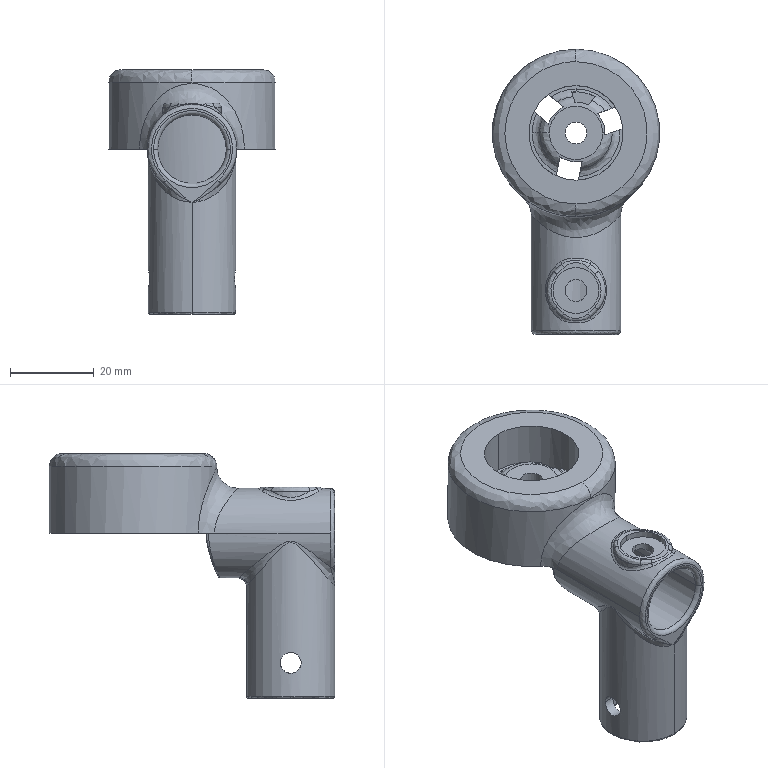Part | SolidWorks | features BaseBody 1 | 1 solid | 251 faces | box 40 x 68.161 x 58.5 mm | volume 24836 mm3 | spline 123 | cylinder 84 | plane 37 | torus 6 | cone 1 | commonest cylinder face diameters 1 x15 34.6 x13 0.986 x12 5 x4 5.2 x4 16.176 x4